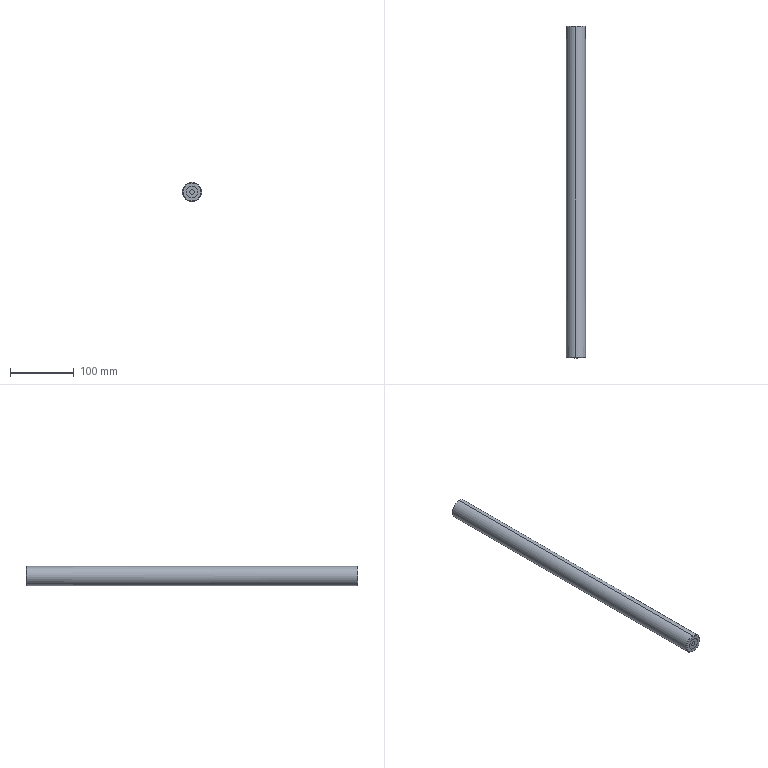Part | SolidWorks | features BaseBody 2 | 2 solids | 17 faces | box 30 x 520 x 30 mm | volume 241731 mm3 | cylinder 8 | plane 5 | cone 4 | commonest cylinder face diameters 18 x4 6.8 x2 30 x2
STEP:
#1=CARTESIAN_POINT('',(0.,-507.,9.));
#2=VERTEX_POINT('',#1);
#3=CARTESIAN_POINT('',(0.,-507.,-9.));
#4=VERTEX_POINT('',#3);
#5=CARTESIAN_POINT('',(0.,-507.,0.));
#6=DIRECTION('',(0.,1.,0.));
#7=DIRECTION('',(0.,0.,1.));
#8=AXIS2_PLACEMENT_3D('',#5,#6,#7);
#9=CIRCLE('',#8,9.);
#10=EDGE_CURVE('',#2,#4,#9,.T.);
#11=ORIENTED_EDGE('',*,*,#10,.T.);
#12=CARTESIAN_POINT('',(0.,-507.,0.));
#13=DIRECTION('',(0.,1.,0.));
#14=DIRECTION('',(0.,0.,1.));
#15=AXIS2_PLACEMENT_3D('',#12,#13,#14);
#16=CIRCLE('',#15,9.);
#17=EDGE_CURVE('',#4,#2,#16,.T.);
#18=ORIENTED_EDGE('',*,*,#17,.T.);
#19=EDGE_LOOP('',(#11,#18));
#20=FACE_OUTER_BOUND('',#19,.T.);
#21=CARTESIAN_POINT('',(0.,-507.,0.));
#22=DIRECTION('',(0.,1.,0.));
#23=DIRECTION('',(1.,0.,0.));
#24=AXIS2_PLACEMENT_3D('',#21,#22,#23);
#25=PLANE('',#24);
#26=ADVANCED_FACE('',(#20),#25,.T.);
#27=CARTESIAN_POINT('',(0.,0.,-9.));
#28=VERTEX_POINT('',#27);
#29=CARTESIAN_POINT('',(0.,-507.,-9.));
#30=DIRECTION('',(0.,1.,0.));
#31=VECTOR('',#30,1000.);
#32=LINE('',#29,#31);
#33=EDGE_CURVE('',#4,#28,#32,.T.);
#34=ORIENTED_EDGE('',*,*,#33,.F.);
#35=ORIENTED_EDGE('',*,*,#10,.F.);
#36=CARTESIAN_POINT('',(0.,0.,9.));
#37=VERTEX_POINT('',#36);
#38=CARTESIAN_POINT('',(0.,-507.,9.));
#39=DIRECTION('',(0.,1.,0.));
#40=VECTOR('',#39,1000.);
#41=LINE('',#38,#40);
#42=EDGE_CURVE('',#2,#37,#41,.T.);
#43=ORIENTED_EDGE('',*,*,#42,.T.);
#44=CARTESIAN_POINT('',(0.,0.,0.));
#45=DIRECTION('',(0.,-1.,0.));
#46=DIRECTION('',(0.,0.,1.));
#47=AXIS2_PLACEMENT_3D('',#44,#45,#46);
#48=CIRCLE('',#47,9.);
#49=EDGE_CURVE('',#28,#37,#48,.T.);
#50=ORIENTED_EDGE('',*,*,#49,.F.);
#51=EDGE_LOOP('',(#34,#35,#43,#50));
#52=FACE_OUTER_BOUND('',#51,.T.);
#53=CARTESIAN_POINT('',(0.,-507.,0.));
#54=DIRECTION('',(0.,1.,0.));
#55=DIRECTION('',(0.,0.,1.));
#56=AXIS2_PLACEMENT_3D('',#53,#54,#55);
#57=CYLINDRICAL_SURFACE('',#56,9.);
#58=ADVANCED_FACE('',(#52),#57,.F.);
#59=CARTESIAN_POINT('',(-14.,-520.,0.));
#60=VERTEX_POINT('',#59);
#61=CARTESIAN_POINT('',(14.,-520.,0.));
#62=VERTEX_POINT('',#61);
#63=CARTESIAN_POINT('',(0.,-520.,0.));
#64=DIRECTION('',(0.,1.,0.));
#65=DIRECTION('',(-1.,0.,0.));
#66=AXIS2_PLACEMENT_3D('',#63,#64,#65);
#67=CIRCLE('',#66,14.);
#68=EDGE_CURVE('',#60,#62,#67,.T.);
#69=ORIENTED_EDGE('',*,*,#68,.F.);
#70=CARTESIAN_POINT('',(0.,-520.,0.));
#71=DIRECTION('',(0.,1.,0.));
#72=DIRECTION('',(-1.,0.,0.));
#73=AXIS2_PLACEMENT_3D('',#70,#71,#72);
#74=CIRCLE('',#73,14.);
#75=EDGE_CURVE('',#62,#60,#74,.T.);
#76=ORIENTED_EDGE('',*,*,#75,.F.);
#77=EDGE_LOOP('',(#69,#76));
#78=FACE_OUTER_BOUND('',#77,.T.);
#79=CARTESIAN_POINT('',(0.,-520.,0.));
#80=DIRECTION('',(0.,1.,0.));
#81=DIRECTION('',(1.,0.,0.));
#82=AXIS2_PLACEMENT_3D('',#79,#80,#81);
#83=PLANE('',#82);
#84=ADVANCED_FACE('',(#78),#83,.F.);
#85=CARTESIAN_POINT('',(0.,0.,0.));
#86=DIRECTION('',(0.,-1.,0.));
#87=DIRECTION('',(0.,0.,1.));
#88=AXIS2_PLACEMENT_3D('',#85,#86,#87);
#89=CIRCLE('',#88,9.);
#90=EDGE_CURVE('',#37,#28,#89,.T.);
#91=ORIENTED_EDGE('',*,*,#90,.T.);
#92=ORIENTED_EDGE('',*,*,#49,.T.);
#93=EDGE_LOOP('',(#91,#92));
#94=FACE_BOUND('',#93,.T.);
#95=CARTESIAN_POINT('',(0.,0.,-14.));
#96=VERTEX_POINT('',#95);
#97=CARTESIAN_POINT('',(0.,0.,14.));
#98=VERTEX_POINT('',#97);
#99=CARTESIAN_POINT('',(0.,0.,0.));
#100=DIRECTION('',(0.,-1.,0.));
#101=DIRECTION('',(0.,0.,-1.));
#102=AXIS2_PLACEMENT_3D('',#99,#100,#101);
#103=CIRCLE('',#102,14.);
#104=EDGE_CURVE('',#96,#98,#103,.T.);
#105=ORIENTED_EDGE('',*,*,#104,.F.);
#106=CARTESIAN_POINT('',(0.,0.,0.));
#107=DIRECTION('',(0.,-1.,0.));
#108=DIRECTION('',(0.,0.,-1.));
#109=AXIS2_PLACEMENT_3D('',#106,#107,#108);
#110=CIRCLE('',#109,14.);
#111=EDGE_CURVE('',#98,#96,#110,.T.);
#112=ORIENTED_EDGE('',*,*,#111,.F.);
#113=EDGE_LOOP('',(#105,#112));
#114=FACE_OUTER_BOUND('',#113,.T.);
#115=CARTESIAN_POINT('',(0.,0.,0.));
#116=DIRECTION('',(0.,1.,0.));
#117=DIRECTION('',(1.,0.,0.));
#118=AXIS2_PLACEMENT_3D('',#115,#116,#117);
#119=PLANE('',#118);
#120=ADVANCED_FACE('',(#94,#114),#119,.T.);
#121=CARTESIAN_POINT('',(15.,-519.,0.));
#122=VERTEX_POINT('',#121);
#123=CARTESIAN_POINT('',(15.,-519.,0.));
#124=DIRECTION('',(0.7071,0.7071,0.));
#125=VECTOR('',#124,1000.);
#126=LINE('',#123,#125);
#127=EDGE_CURVE('',#62,#122,#126,.T.);
#128=ORIENTED_EDGE('',*,*,#127,.F.);
#129=ORIENTED_EDGE('',*,*,#75,.T.);
#130=CARTESIAN_POINT('',(-15.,-519.,0.));
#131=VERTEX_POINT('',#130);
#132=CARTESIAN_POINT('',(-15.,-519.,0.));
#133=DIRECTION('',(-0.7071,0.7071,0.));
#134=VECTOR('',#133,1000.);
#135=LINE('',#132,#134);
#136=EDGE_CURVE('',#60,#131,#135,.T.);
#137=ORIENTED_EDGE('',*,*,#136,.T.);
#138=CARTESIAN_POINT('',(0.,-519.,-15.));
#139=VERTEX_POINT('',#138);
#140=CARTESIAN_POINT('',(0.,-519.,0.));
#141=DIRECTION('',(0.,1.,0.));
#142=DIRECTION('',(0.,0.,1.));
#143=AXIS2_PLACEMENT_3D('',#140,#141,#142);
#144=CIRCLE('',#143,15.);
#145=EDGE_CURVE('',#139,#131,#144,.T.);
#146=ORIENTED_EDGE('',*,*,#145,.F.);
#147=CARTESIAN_POINT('',(0.,-519.,0.));
#148=DIRECTION('',(0.,1.,0.));
#149=DIRECTION('',(0.,0.,1.));
#150=AXIS2_PLACEMENT_3D('',#147,#148,#149);
#151=CIRCLE('',#150,15.);
#152=EDGE_CURVE('',#122,#139,#151,.T.);
#153=ORIENTED_EDGE('',*,*,#152,.F.);
#154=EDGE_LOOP('',(#128,#129,#137,#146,#153));
#155=FACE_OUTER_BOUND('',#154,.T.);
#156=CARTESIAN_POINT('',(0.,-519.,0.));
#157=DIRECTION('',(0.,1.,0.));
#158=DIRECTION('',(-1.,0.,0.));
#159=AXIS2_PLACEMENT_3D('',#156,#157,#158);
#160=CONICAL_SURFACE('',#159,15.,0.7854);
#161=ADVANCED_FACE('',(#155),#160,.T.);
#162=CARTESIAN_POINT('',(0.,-1.,15.));
#163=VERTEX_POINT('',#162);
#164=CARTESIAN_POINT('',(0.,-1.,15.));
#165=DIRECTION('',(0.,-0.7071,0.7071));
#166=VECTOR('',#165,1000.);
#167=LINE('',#164,#166);
#168=EDGE_CURVE('',#98,#163,#167,.T.);
#169=ORIENTED_EDGE('',*,*,#168,.F.);
#170=ORIENTED_EDGE('',*,*,#111,.T.);
#171=CARTESIAN_POINT('',(0.,-1.,-15.));
#172=VERTEX_POINT('',#171);
#173=CARTESIAN_POINT('',(0.,-1.,-15.));
#174=DIRECTION('',(0.,-0.7071,-0.7071));
#175=VECTOR('',#174,1000.);
#176=LINE('',#173,#175);
#177=EDGE_CURVE('',#96,#172,#176,.T.);
#178=ORIENTED_EDGE('',*,*,#177,.T.);
#179=CARTESIAN_POINT('',(0.,-1.,0.));
#180=DIRECTION('',(0.,-1.,0.));
#181=DIRECTION('',(0.,0.,1.));
#182=AXIS2_PLACEMENT_3D('',#179,#180,#181);
#183=CIRCLE('',#182,15.);
#184=EDGE_CURVE('',#163,#172,#183,.T.);
#185=ORIENTED_EDGE('',*,*,#184,.F.);
#186=EDGE_LOOP('',(#169,#170,#178,#185));
#187=FACE_OUTER_BOUND('',#186,.T.);
#188=CARTESIAN_POINT('',(0.,-1.,0.));
#189=DIRECTION('',(0.,-1.,0.));
#190=DIRECTION('',(0.,0.,-1.));
#191=AXIS2_PLACEMENT_3D('',#188,#189,#190);
#192=CONICAL_SURFACE('',#191,15.,0.7854);
#193=ADVANCED_FACE('',(#187),#192,.T.);
#194=CARTESIAN_POINT('',(0.,-520.,-15.));
#195=DIRECTION('',(0.,1.,0.));
#196=VECTOR('',#195,1000.);
#197=LINE('',#194,#196);
#198=EDGE_CURVE('',#139,#172,#197,.T.);
#199=ORIENTED_EDGE('',*,*,#198,.F.);
#200=ORIENTED_EDGE('',*,*,#145,.T.);
#201=CARTESIAN_POINT('',(0.,-519.,15.));
#202=VERTEX_POINT('',#201);
#203=CARTESIAN_POINT('',(0.,-519.,0.));
#204=DIRECTION('',(0.,1.,0.));
#205=DIRECTION('',(0.,0.,1.));
#206=AXIS2_PLACEMENT_3D('',#203,#204,#205);
#207=CIRCLE('',#206,15.);
#208=EDGE_CURVE('',#131,#202,#207,.T.);
#209=ORIENTED_EDGE('',*,*,#208,.T.);
#210=CARTESIAN_POINT('',(0.,-520.,15.));
#211=DIRECTION('',(0.,1.,0.));
#212=VECTOR('',#211,1000.);
#213=LINE('',#210,#212);
#214=EDGE_CURVE('',#202,#163,#213,.T.);
#215=ORIENTED_EDGE('',*,*,#214,.T.);
#216=ORIENTED_EDGE('',*,*,#184,.T.);
#217=EDGE_LOOP('',(#199,#200,#209,#215,#216));
#218=FACE_OUTER_BOUND('',#217,.T.);
#219=CARTESIAN_POINT('',(0.,-520.,0.));
#220=DIRECTION('',(0.,1.,0.));
#221=DIRECTION('',(0.,0.,1.));
#222=AXIS2_PLACEMENT_3D('',#219,#220,#221);
#223=CYLINDRICAL_SURFACE('',#222,15.);
#224=ADVANCED_FACE('',(#218),#223,.T.);
#225=ORIENTED_EDGE('',*,*,#17,.F.);
#226=ORIENTED_EDGE('',*,*,#33,.T.);
#227=ORIENTED_EDGE('',*,*,#90,.F.);
#228=ORIENTED_EDGE('',*,*,#42,.F.);
#229=EDGE_LOOP('',(#225,#226,#227,#228));
#230=FACE_OUTER_BOUND('',#229,.T.);
#231=CARTESIAN_POINT('',(0.,-507.,0.));
#232=DIRECTION('',(0.,1.,0.));
#233=DIRECTION('',(0.,0.,1.));
#234=AXIS2_PLACEMENT_3D('',#231,#232,#233);
#235=CYLINDRICAL_SURFACE('',#234,9.);
#236=ADVANCED_FACE('',(#230),#235,.F.);
#237=ORIENTED_EDGE('',*,*,#68,.T.);
#238=ORIENTED_EDGE('',*,*,#127,.T.);
#239=CARTESIAN_POINT('',(0.,-519.,0.));
#240=DIRECTION('',(0.,1.,0.));
#241=DIRECTION('',(0.,0.,1.));
#242=AXIS2_PLACEMENT_3D('',#239,#240,#241);
#243=CIRCLE('',#242,15.);
#244=EDGE_CURVE('',#202,#122,#243,.T.);
#245=ORIENTED_EDGE('',*,*,#244,.F.);
#246=ORIENTED_EDGE('',*,*,#208,.F.);
#247=ORIENTED_EDGE('',*,*,#136,.F.);
#248=EDGE_LOOP('',(#237,#238,#245,#246,#247));
#249=FACE_OUTER_BOUND('',#248,.T.);
#250=CARTESIAN_POINT('',(0.,-519.,0.));
#251=DIRECTION('',(0.,1.,0.));
#252=DIRECTION('',(-1.,0.,0.));
#253=AXIS2_PLACEMENT_3D('',#250,#251,#252);
#254=CONICAL_SURFACE('',#253,15.,0.7854);
#255=ADVANCED_FACE('',(#249),#254,.T.);
#256=ORIENTED_EDGE('',*,*,#104,.T.);
#257=ORIENTED_EDGE('',*,*,#168,.T.);
#258=CARTESIAN_POINT('',(0.,-1.,0.));
#259=DIRECTION('',(0.,-1.,0.));
#260=DIRECTION('',(0.,0.,1.));
#261=AXIS2_PLACEMENT_3D('',#258,#259,#260);
#262=CIRCLE('',#261,15.);
#263=EDGE_CURVE('',#172,#163,#262,.T.);
#264=ORIENTED_EDGE('',*,*,#263,.F.);
#265=ORIENTED_EDGE('',*,*,#177,.F.);
#266=EDGE_LOOP('',(#256,#257,#264,#265));
#267=FACE_OUTER_BOUND('',#266,.T.);
#268=CARTESIAN_POINT('',(0.,-1.,0.));
#269=DIRECTION('',(0.,-1.,0.));
#270=DIRECTION('',(0.,0.,-1.));
#271=AXIS2_PLACEMENT_3D('',#268,#269,#270);
#272=CONICAL_SURFACE('',#271,15.,0.7854);
#273=ADVANCED_FACE('',(#267),#272,.T.);
#274=ORIENTED_EDGE('',*,*,#152,.T.);
#275=ORIENTED_EDGE('',*,*,#198,.T.);
#276=ORIENTED_EDGE('',*,*,#263,.T.);
#277=ORIENTED_EDGE('',*,*,#214,.F.);
#278=ORIENTED_EDGE('',*,*,#244,.T.);
#279=EDGE_LOOP('',(#274,#275,#276,#277,#278));
#280=FACE_OUTER_BOUND('',#279,.T.);
#281=CARTESIAN_POINT('',(0.,-520.,0.));
#282=DIRECTION('',(0.,1.,0.));
#283=DIRECTION('',(0.,0.,1.));
#284=AXIS2_PLACEMENT_3D('',#281,#282,#283);
#285=CYLINDRICAL_SURFACE('',#284,15.);
#286=ADVANCED_FACE('',(#280),#285,.T.);
#287=CLOSED_SHELL('',(#26,#58,#84,#120,#161,#193,#224,#236,#255,#273,#286));
#288=MANIFOLD_SOLID_BREP('',#287);
#289=CARTESIAN_POINT('',(0.,-505.,3.4));
#290=VERTEX_POINT('',#289);
#291=CARTESIAN_POINT('',(0.,-520.,3.4));
#292=VERTEX_POINT('',#291);
#293=CARTESIAN_POINT('',(0.,-520.,3.4));
#294=DIRECTION('',(0.,-1.,0.));
#295=VECTOR('',#294,1000.);
#296=LINE('',#293,#295);
#297=EDGE_CURVE('',#290,#292,#296,.T.);
#298=ORIENTED_EDGE('',*,*,#297,.F.);
#299=CARTESIAN_POINT('',(0.,-505.,-3.4));
#300=VERTEX_POINT('',#299);
#301=CARTESIAN_POINT('',(0.,-505.,0.));
#302=DIRECTION('',(0.,1.,0.));
#303=DIRECTION('',(0.,0.,-1.));
#304=AXIS2_PLACEMENT_3D('',#301,#302,#303);
#305=CIRCLE('',#304,3.4);
#306=EDGE_CURVE('',#290,#300,#305,.T.);
#307=ORIENTED_EDGE('',*,*,#306,.T.);
#308=CARTESIAN_POINT('',(0.,-520.,-3.4));
#309=VERTEX_POINT('',#308);
#310=CARTESIAN_POINT('',(0.,-520.,-3.4));
#311=DIRECTION('',(0.,-1.,0.));
#312=VECTOR('',#311,1000.);
#313=LINE('',#310,#312);
#314=EDGE_CURVE('',#300,#309,#313,.T.);
#315=ORIENTED_EDGE('',*,*,#314,.T.);
#316=CARTESIAN_POINT('',(0.,-520.,0.));
#317=DIRECTION('',(0.,1.,0.));
#318=DIRECTION('',(0.,0.,-1.));
#319=AXIS2_PLACEMENT_3D('',#316,#317,#318);
#320=CIRCLE('',#319,3.4);
#321=EDGE_CURVE('',#292,#309,#320,.T.);
#322=ORIENTED_EDGE('',*,*,#321,.F.);
#323=EDGE_LOOP('',(#298,#307,#315,#322));
#324=FACE_OUTER_BOUND('',#323,.T.);
#325=CARTESIAN_POINT('',(0.,-520.,0.));
#326=DIRECTION('',(0.,-1.,0.));
#327=DIRECTION('',(0.,0.,-1.));
#328=AXIS2_PLACEMENT_3D('',#325,#326,#327);
#329=CYLINDRICAL_SURFACE('',#328,3.4);
#330=ADVANCED_FACE('',(#324),#329,.F.);
#331=CARTESIAN_POINT('',(0.,-505.,0.));
#332=DIRECTION('',(0.,1.,0.));
#333=DIRECTION('',(0.,0.,-1.));
#334=AXIS2_PLACEMENT_3D('',#331,#332,#333);
#335=CIRCLE('',#334,3.4);
#336=EDGE_CURVE('',#300,#290,#335,.T.);
#337=ORIENTED_EDGE('',*,*,#336,.F.);
#338=ORIENTED_EDGE('',*,*,#306,.F.);
#339=EDGE_LOOP('',(#337,#338));
#340=FACE_BOUND('',#339,.T.);
#341=CARTESIAN_POINT('',(0.,-505.,-9.));
#342=VERTEX_POINT('',#341);
#343=CARTESIAN_POINT('',(0.,-505.,9.));
#344=VERTEX_POINT('',#343);
#345=CARTESIAN_POINT('',(0.,-505.,0.));
#346=DIRECTION('',(0.,-1.,0.));
#347=DIRECTION('',(0.,0.,-1.));
#348=AXIS2_PLACEMENT_3D('',#345,#346,#347);
#349=CIRCLE('',#348,9.);
#350=EDGE_CURVE('',#342,#344,#349,.T.);
#351=ORIENTED_EDGE('',*,*,#350,.F.);
#352=CARTESIAN_POINT('',(0.,-505.,0.));
#353=DIRECTION('',(0.,-1.,0.));
#354=DIRECTION('',(0.,0.,-1.));
#355=AXIS2_PLACEMENT_3D('',#352,#353,#354);
#356=CIRCLE('',#355,9.);
#357=EDGE_CURVE('',#344,#342,#356,.T.);
#358=ORIENTED_EDGE('',*,*,#357,.F.);
#359=EDGE_LOOP('',(#351,#358));
#360=FACE_OUTER_BOUND('',#359,.T.);
#361=CARTESIAN_POINT('',(0.,-505.,0.));
#362=DIRECTION('',(0.,-1.,0.));
#363=DIRECTION('',(0.,0.,-1.));
#364=AXIS2_PLACEMENT_3D('',#361,#362,#363);
#365=PLANE('',#364);
#366=ADVANCED_FACE('',(#340,#360),#365,.F.);
#367=CARTESIAN_POINT('',(0.,-520.,0.));
#368=DIRECTION('',(0.,1.,0.));
#369=DIRECTION('',(0.,0.,-1.));
#370=AXIS2_PLACEMENT_3D('',#367,#368,#369);
#371=CIRCLE('',#370,3.4);
#372=EDGE_CURVE('',#309,#292,#371,.T.);
#373=ORIENTED_EDGE('',*,*,#372,.T.);
#374=ORIENTED_EDGE('',*,*,#321,.T.);
#375=EDGE_LOOP('',(#373,#374));
#376=FACE_BOUND('',#375,.T.);
#377=CARTESIAN_POINT('',(0.,-520.,-9.));
#378=VERTEX_POINT('',#377);
#379=CARTESIAN_POINT('',(0.,-520.,9.));
#380=VERTEX_POINT('',#379);
#381=CARTESIAN_POINT('',(0.,-520.,0.));
#382=DIRECTION('',(0.,1.,0.));
#383=DIRECTION('',(0.,0.,-1.));
#384=AXIS2_PLACEMENT_3D('',#381,#382,#383);
#385=CIRCLE('',#384,9.);
#386=EDGE_CURVE('',#378,#380,#385,.T.);
#387=ORIENTED_EDGE('',*,*,#386,.F.);
#388=CARTESIAN_POINT('',(0.,-520.,0.));
#389=DIRECTION('',(0.,1.,0.));
#390=DIRECTION('',(0.,0.,-1.));
#391=AXIS2_PLACEMENT_3D('',#388,#389,#390);
#392=CIRCLE('',#391,9.);
#393=EDGE_CURVE('',#380,#378,#392,.T.);
#394=ORIENTED_EDGE('',*,*,#393,.F.);
#395=EDGE_LOOP('',(#387,#394));
#396=FACE_OUTER_BOUND('',#395,.T.);
#397=CARTESIAN_POINT('',(0.,-520.,0.));
#398=DIRECTION('',(0.,-1.,0.));
#399=DIRECTION('',(0.,0.,-1.));
#400=AXIS2_PLACEMENT_3D('',#397,#398,#399);
#401=PLANE('',#400);
#402=ADVANCED_FACE('',(#376,#396),#401,.T.);
#403=CARTESIAN_POINT('',(0.,-505.,9.));
#404=DIRECTION('',(0.,-1.,0.));
#405=VECTOR('',#404,1000.);
#406=LINE('',#403,#405);
#407=EDGE_CURVE('',#344,#380,#406,.T.);
#408=ORIENTED_EDGE('',*,*,#407,.F.);
#409=ORIENTED_EDGE('',*,*,#357,.T.);
#410=CARTESIAN_POINT('',(0.,-505.,-9.));
#411=DIRECTION('',(0.,-1.,0.));
#412=VECTOR('',#411,1000.);
#413=LINE('',#410,#412);
#414=EDGE_CURVE('',#342,#378,#413,.T.);
#415=ORIENTED_EDGE('',*,*,#414,.T.);
#416=ORIENTED_EDGE('',*,*,#386,.T.);
#417=EDGE_LOOP('',(#408,#409,#415,#416));
#418=FACE_OUTER_BOUND('',#417,.T.);
#419=CARTESIAN_POINT('',(0.,-505.,0.));
#420=DIRECTION('',(0.,-1.,0.));
#421=DIRECTION('',(0.,0.,-1.));
#422=AXIS2_PLACEMENT_3D('',#419,#420,#421);
#423=CYLINDRICAL_SURFACE('',#422,9.);
#424=ADVANCED_FACE('',(#418),#423,.T.);
#425=ORIENTED_EDGE('',*,*,#336,.T.);
#426=ORIENTED_EDGE('',*,*,#297,.T.);
#427=ORIENTED_EDGE('',*,*,#372,.F.);
#428=ORIENTED_EDGE('',*,*,#314,.F.);
#429=EDGE_LOOP('',(#425,#426,#427,#428));
#430=FACE_OUTER_BOUND('',#429,.T.);
#431=CARTESIAN_POINT('',(0.,-520.,0.));
#432=DIRECTION('',(0.,-1.,0.));
#433=DIRECTION('',(0.,0.,-1.));
#434=AXIS2_PLACEMENT_3D('',#431,#432,#433);
#435=CYLINDRICAL_SURFACE('',#434,3.4);
#436=ADVANCED_FACE('',(#430),#435,.F.);
#437=ORIENTED_EDGE('',*,*,#350,.T.);
#438=ORIENTED_EDGE('',*,*,#407,.T.);
#439=ORIENTED_EDGE('',*,*,#393,.T.);
#440=ORIENTED_EDGE('',*,*,#414,.F.);
#441=EDGE_LOOP('',(#437,#438,#439,#440));
#442=FACE_OUTER_BOUND('',#441,.T.);
#443=CARTESIAN_POINT('',(0.,-505.,0.));
#444=DIRECTION('',(0.,-1.,0.));
#445=DIRECTION('',(0.,0.,-1.));
#446=AXIS2_PLACEMENT_3D('',#443,#444,#445);
#447=CYLINDRICAL_SURFACE('',#446,9.);
#448=ADVANCED_FACE('',(#442),#447,.T.);
#449=CLOSED_SHELL('',(#330,#366,#402,#424,#436,#448));
#450=MANIFOLD_SOLID_BREP('',#449);
#451=CARTESIAN_POINT('',(0.,0.,0.));
#452=DIRECTION('',(0.,0.,1.));
#453=DIRECTION('',(1.,0.,0.));
#454=AXIS2_PLACEMENT_3D('',#451,#452,#453);
#455=(LENGTH_UNIT()NAMED_UNIT(*)SI_UNIT(.MILLI.,.METRE.));
#456=UNCERTAINTY_MEASURE_WITH_UNIT(LENGTH_MEASURE(0.00001),#455,'','');
#457=(NAMED_UNIT(*)PLANE_ANGLE_UNIT()SI_UNIT($,.RADIAN.));
#458=(NAMED_UNIT(*)SI_UNIT($,.STERADIAN.)SOLID_ANGLE_UNIT());
#459=(GEOMETRIC_REPRESENTATION_CONTEXT(3)GLOBAL_UNCERTAINTY_ASSIGNED_CONTEXT((#456))GLOBAL_UNIT_ASSIGNED_CONTEXT((#455,#457,#458))REPRESENTATION_CONTEXT('',''));
#460=ADVANCED_BREP_SHAPE_REPRESENTATION('',(#288,#450,#454),#459);